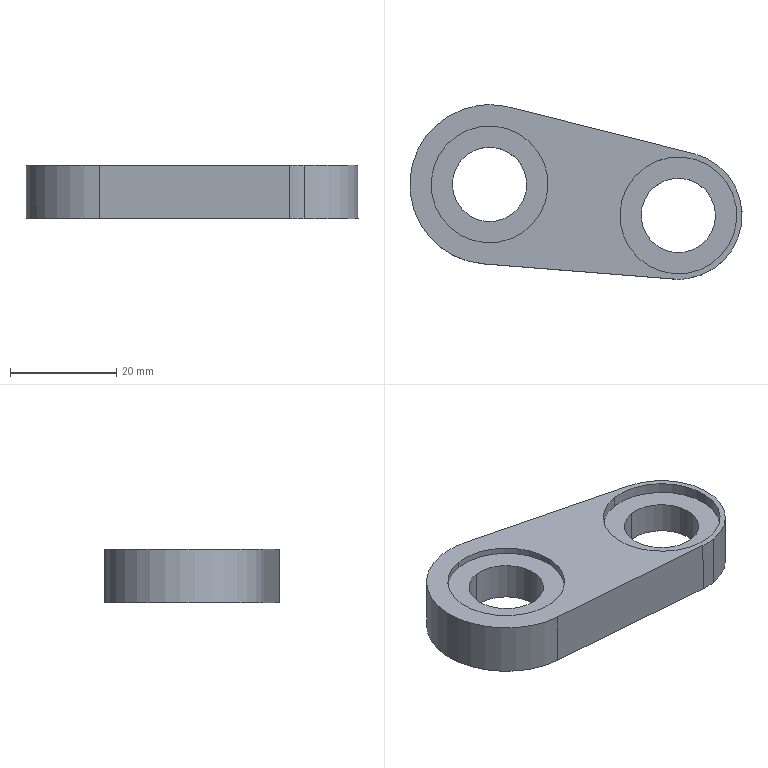Part | SolidWorks | features BaseBody 1 | 1 solid | 24 faces | box 62.525 x 32.838 x 10.009 mm | volume 10933 mm3 | cylinder 16 | plane 8 | commonest cylinder face diameters 22 x8 14 x4 24 x2 30 x2
STEP:
#1=CARTESIAN_POINT('',(378.377,184.65,13.48));
#2=VERTEX_POINT('',#1);
#3=CARTESIAN_POINT('',(376.21,198.481,13.48));
#4=VERTEX_POINT('',#3);
#5=CARTESIAN_POINT('',(377.293,191.566,13.48));
#6=DIRECTION('',(0.0001435,0.000000521,-1.));
#7=DIRECTION('',(1.,0.,0.0001435));
#8=AXIS2_PLACEMENT_3D('',#5,#6,#7);
#9=CIRCLE('',#8,7.);
#10=EDGE_CURVE('',#2,#4,#9,.T.);
#11=ORIENTED_EDGE('',*,*,#10,.F.);
#12=CARTESIAN_POINT('',(378.377,184.65,7.48));
#13=VERTEX_POINT('',#12);
#14=CARTESIAN_POINT('',(378.376,184.65,15.48));
#15=DIRECTION('',(0.0001435,0.000000521,-1.));
#16=VECTOR('',#15,1000.);
#17=LINE('',#14,#16);
#18=EDGE_CURVE('',#2,#13,#17,.T.);
#19=ORIENTED_EDGE('',*,*,#18,.T.);
#20=CARTESIAN_POINT('',(376.211,198.481,7.48));
#21=VERTEX_POINT('',#20);
#22=CARTESIAN_POINT('',(377.294,191.566,7.48));
#23=DIRECTION('',(-0.0001435,-0.000000521,1.));
#24=DIRECTION('',(0.1548,-0.988,0.00002169));
#25=AXIS2_PLACEMENT_3D('',#22,#23,#24);
#26=CIRCLE('',#25,7.);
#27=EDGE_CURVE('',#21,#13,#26,.T.);
#28=ORIENTED_EDGE('',*,*,#27,.F.);
#29=CARTESIAN_POINT('',(376.21,198.481,15.48));
#30=DIRECTION('',(0.0001435,0.000000521,-1.));
#31=VECTOR('',#30,1000.);
#32=LINE('',#29,#31);
#33=EDGE_CURVE('',#4,#21,#32,.T.);
#34=ORIENTED_EDGE('',*,*,#33,.F.);
#35=EDGE_LOOP('',(#11,#19,#28,#34));
#36=FACE_OUTER_BOUND('',#35,.T.);
#37=CARTESIAN_POINT('',(377.293,191.566,15.48));
#38=DIRECTION('',(0.0001435,0.000000521,-1.));
#39=DIRECTION('',(-0.1548,0.988,-0.00002169));
#40=AXIS2_PLACEMENT_3D('',#37,#38,#39);
#41=CYLINDRICAL_SURFACE('',#40,7.);
#42=ADVANCED_FACE('',(#36),#41,.F.);
#43=CARTESIAN_POINT('',(375.591,202.433,13.479));
#44=VERTEX_POINT('',#43);
#45=CARTESIAN_POINT('',(378.996,180.698,13.48));
#46=VERTEX_POINT('',#45);
#47=CARTESIAN_POINT('',(377.293,191.566,13.48));
#48=DIRECTION('',(-0.0001435,-0.000000521,1.));
#49=DIRECTION('',(0.1548,-0.988,0.00002169));
#50=AXIS2_PLACEMENT_3D('',#47,#48,#49);
#51=CIRCLE('',#50,11.);
#52=EDGE_CURVE('',#44,#46,#51,.T.);
#53=ORIENTED_EDGE('',*,*,#52,.F.);
#54=CARTESIAN_POINT('',(375.59,202.433,15.479));
#55=VERTEX_POINT('',#54);
#56=CARTESIAN_POINT('',(375.591,202.433,14.279));
#57=DIRECTION('',(-0.0001435,-0.000000521,1.));
#58=VECTOR('',#57,1000.);
#59=LINE('',#56,#58);
#60=EDGE_CURVE('',#44,#55,#59,.T.);
#61=ORIENTED_EDGE('',*,*,#60,.T.);
#62=CARTESIAN_POINT('',(378.995,180.698,15.48));
#63=VERTEX_POINT('',#62);
#64=CARTESIAN_POINT('',(377.293,191.566,15.48));
#65=DIRECTION('',(0.0001435,0.000000521,-1.));
#66=DIRECTION('',(-1.,0.,-0.0001435));
#67=AXIS2_PLACEMENT_3D('',#64,#65,#66);
#68=CIRCLE('',#67,11.);
#69=EDGE_CURVE('',#63,#55,#68,.T.);
#70=ORIENTED_EDGE('',*,*,#69,.F.);
#71=CARTESIAN_POINT('',(378.996,180.698,14.28));
#72=DIRECTION('',(-0.0001435,-0.000000521,1.));
#73=VECTOR('',#72,1000.);
#74=LINE('',#71,#73);
#75=EDGE_CURVE('',#46,#63,#74,.T.);
#76=ORIENTED_EDGE('',*,*,#75,.F.);
#77=EDGE_LOOP('',(#53,#61,#70,#76));
#78=FACE_OUTER_BOUND('',#77,.T.);
#79=CARTESIAN_POINT('',(377.293,191.566,14.28));
#80=DIRECTION('',(-0.0001435,-0.000000521,1.));
#81=DIRECTION('',(0.1548,-0.988,0.00002169));
#82=AXIS2_PLACEMENT_3D('',#79,#80,#81);
#83=CYLINDRICAL_SURFACE('',#82,11.);
#84=ADVANCED_FACE('',(#78),#83,.F.);
#85=CARTESIAN_POINT('',(340.067,208.271,14.274));
#86=VERTEX_POINT('',#85);
#87=CARTESIAN_POINT('',(343.472,186.536,14.275));
#88=VERTEX_POINT('',#87);
#89=CARTESIAN_POINT('',(341.77,197.404,14.275));
#90=DIRECTION('',(-0.0001435,-0.000000521,1.));
#91=DIRECTION('',(1.,0.,0.0001435));
#92=AXIS2_PLACEMENT_3D('',#89,#90,#91);
#93=CIRCLE('',#92,11.);
#94=EDGE_CURVE('',#86,#88,#93,.T.);
#95=ORIENTED_EDGE('',*,*,#94,.F.);
#96=CARTESIAN_POINT('',(340.067,208.271,15.474));
#97=VERTEX_POINT('',#96);
#98=CARTESIAN_POINT('',(340.067,208.271,14.274));
#99=DIRECTION('',(-0.0001435,-0.000000521,1.));
#100=VECTOR('',#99,1000.);
#101=LINE('',#98,#100);
#102=EDGE_CURVE('',#86,#97,#101,.T.);
#103=ORIENTED_EDGE('',*,*,#102,.T.);
#104=CARTESIAN_POINT('',(343.472,186.536,15.475));
#105=VERTEX_POINT('',#104);
#106=CARTESIAN_POINT('',(341.769,197.404,15.475));
#107=DIRECTION('',(0.0001435,0.000000521,-1.));
#108=DIRECTION('',(0.1548,-0.988,0.00002169));
#109=AXIS2_PLACEMENT_3D('',#106,#107,#108);
#110=CIRCLE('',#109,11.);
#111=EDGE_CURVE('',#105,#97,#110,.T.);
#112=ORIENTED_EDGE('',*,*,#111,.F.);
#113=CARTESIAN_POINT('',(343.472,186.536,14.275));
#114=DIRECTION('',(-0.0001435,-0.000000521,1.));
#115=VECTOR('',#114,1000.);
#116=LINE('',#113,#115);
#117=EDGE_CURVE('',#88,#105,#116,.T.);
#118=ORIENTED_EDGE('',*,*,#117,.F.);
#119=EDGE_LOOP('',(#95,#103,#112,#118));
#120=FACE_OUTER_BOUND('',#119,.T.);
#121=CARTESIAN_POINT('',(341.77,197.404,14.275));
#122=DIRECTION('',(-0.0001435,-0.000000521,1.));
#123=DIRECTION('',(0.1548,-0.988,0.00002169));
#124=AXIS2_PLACEMENT_3D('',#121,#122,#123);
#125=CYLINDRICAL_SURFACE('',#124,11.);
#126=ADVANCED_FACE('',(#120),#125,.F.);
#127=CARTESIAN_POINT('',(342.853,190.488,14.275));
#128=VERTEX_POINT('',#127);
#129=CARTESIAN_POINT('',(340.686,204.319,14.274));
#130=VERTEX_POINT('',#129);
#131=CARTESIAN_POINT('',(341.77,197.404,14.275));
#132=DIRECTION('',(0.0001435,0.000000521,-1.));
#133=DIRECTION('',(-0.1548,0.988,-0.00002169));
#134=AXIS2_PLACEMENT_3D('',#131,#132,#133);
#135=CIRCLE('',#134,7.);
#136=EDGE_CURVE('',#128,#130,#135,.T.);
#137=ORIENTED_EDGE('',*,*,#136,.F.);
#138=CARTESIAN_POINT('',(342.854,190.488,7.075));
#139=VERTEX_POINT('',#138);
#140=CARTESIAN_POINT('',(342.853,190.488,14.275));
#141=DIRECTION('',(0.0001435,0.000000521,-1.));
#142=VECTOR('',#141,1000.);
#143=LINE('',#140,#142);
#144=EDGE_CURVE('',#128,#139,#143,.T.);
#145=ORIENTED_EDGE('',*,*,#144,.T.);
#146=CARTESIAN_POINT('',(340.687,204.319,7.074));
#147=VERTEX_POINT('',#146);
#148=CARTESIAN_POINT('',(341.771,197.404,7.075));
#149=DIRECTION('',(-0.0001435,-0.000000521,1.));
#150=DIRECTION('',(-0.1548,0.988,-0.00002169));
#151=AXIS2_PLACEMENT_3D('',#148,#149,#150);
#152=CIRCLE('',#151,7.);
#153=EDGE_CURVE('',#147,#139,#152,.T.);
#154=ORIENTED_EDGE('',*,*,#153,.F.);
#155=CARTESIAN_POINT('',(340.686,204.319,14.274));
#156=DIRECTION('',(0.0001435,0.000000521,-1.));
#157=VECTOR('',#156,1000.);
#158=LINE('',#155,#157);
#159=EDGE_CURVE('',#130,#147,#158,.T.);
#160=ORIENTED_EDGE('',*,*,#159,.F.);
#161=EDGE_LOOP('',(#137,#145,#154,#160));
#162=FACE_OUTER_BOUND('',#161,.T.);
#163=CARTESIAN_POINT('',(341.77,197.404,14.275));
#164=DIRECTION('',(0.0001435,0.000000521,-1.));
#165=DIRECTION('',(-0.1548,0.988,-0.00002169));
#166=AXIS2_PLACEMENT_3D('',#163,#164,#165);
#167=CYLINDRICAL_SURFACE('',#166,7.);
#168=ADVANCED_FACE('',(#162),#167,.F.);
#169=CARTESIAN_POINT('',(340.068,208.271,7.074));
#170=VERTEX_POINT('',#169);
#171=CARTESIAN_POINT('',(343.473,186.536,7.075));
#172=VERTEX_POINT('',#171);
#173=CARTESIAN_POINT('',(341.771,197.404,7.075));
#174=DIRECTION('',(0.0001435,0.000000521,-1.));
#175=DIRECTION('',(-0.1548,0.988,-0.00002169));
#176=AXIS2_PLACEMENT_3D('',#173,#174,#175);
#177=CIRCLE('',#176,11.);
#178=EDGE_CURVE('',#170,#172,#177,.T.);
#179=ORIENTED_EDGE('',*,*,#178,.F.);
#180=CARTESIAN_POINT('',(340.068,208.271,5.474));
#181=VERTEX_POINT('',#180);
#182=CARTESIAN_POINT('',(340.068,208.271,7.074));
#183=DIRECTION('',(0.0001435,0.000000521,-1.));
#184=VECTOR('',#183,1000.);
#185=LINE('',#182,#184);
#186=EDGE_CURVE('',#170,#181,#185,.T.);
#187=ORIENTED_EDGE('',*,*,#186,.T.);
#188=CARTESIAN_POINT('',(343.473,186.536,5.475));
#189=VERTEX_POINT('',#188);
#190=CARTESIAN_POINT('',(341.771,197.404,5.475));
#191=DIRECTION('',(-0.0001435,-0.000000521,1.));
#192=DIRECTION('',(-1.,0.,-0.0001435));
#193=AXIS2_PLACEMENT_3D('',#190,#191,#192);
#194=CIRCLE('',#193,11.);
#195=EDGE_CURVE('',#189,#181,#194,.T.);
#196=ORIENTED_EDGE('',*,*,#195,.F.);
#197=CARTESIAN_POINT('',(343.473,186.536,7.075));
#198=DIRECTION('',(0.0001435,0.000000521,-1.));
#199=VECTOR('',#198,1000.);
#200=LINE('',#197,#199);
#201=EDGE_CURVE('',#172,#189,#200,.T.);
#202=ORIENTED_EDGE('',*,*,#201,.F.);
#203=EDGE_LOOP('',(#179,#187,#196,#202));
#204=FACE_OUTER_BOUND('',#203,.T.);
#205=CARTESIAN_POINT('',(341.771,197.404,7.075));
#206=DIRECTION('',(0.0001435,0.000000521,-1.));
#207=DIRECTION('',(0.1548,-0.988,0.00002169));
#208=AXIS2_PLACEMENT_3D('',#205,#206,#207);
#209=CYLINDRICAL_SURFACE('',#208,11.);
#210=ADVANCED_FACE('',(#204),#209,.F.);
#211=CARTESIAN_POINT('',(375.592,202.433,7.479));
#212=VERTEX_POINT('',#211);
#213=CARTESIAN_POINT('',(378.997,180.698,7.48));
#214=VERTEX_POINT('',#213);
#215=CARTESIAN_POINT('',(377.294,191.566,7.48));
#216=DIRECTION('',(0.0001435,0.000000521,-1.));
#217=DIRECTION('',(-0.1548,0.988,-0.00002169));
#218=AXIS2_PLACEMENT_3D('',#215,#216,#217);
#219=CIRCLE('',#218,11.);
#220=EDGE_CURVE('',#212,#214,#219,.T.);
#221=ORIENTED_EDGE('',*,*,#220,.F.);
#222=CARTESIAN_POINT('',(375.592,202.433,5.479));
#223=VERTEX_POINT('',#222);
#224=CARTESIAN_POINT('',(375.592,202.433,7.079));
#225=DIRECTION('',(0.0001435,0.000000521,-1.));
#226=VECTOR('',#225,1000.);
#227=LINE('',#224,#226);
#228=EDGE_CURVE('',#212,#223,#227,.T.);
#229=ORIENTED_EDGE('',*,*,#228,.T.);
#230=CARTESIAN_POINT('',(378.997,180.698,5.48));
#231=VERTEX_POINT('',#230);
#232=CARTESIAN_POINT('',(377.294,191.566,5.48));
#233=DIRECTION('',(-0.0001435,-0.000000521,1.));
#234=DIRECTION('',(0.1548,-0.988,0.00002169));
#235=AXIS2_PLACEMENT_3D('',#232,#233,#234);
#236=CIRCLE('',#235,11.);
#237=EDGE_CURVE('',#231,#223,#236,.T.);
#238=ORIENTED_EDGE('',*,*,#237,.F.);
#239=CARTESIAN_POINT('',(378.997,180.698,7.08));
#240=DIRECTION('',(0.0001435,0.000000521,-1.));
#241=VECTOR('',#240,1000.);
#242=LINE('',#239,#241);
#243=EDGE_CURVE('',#214,#231,#242,.T.);
#244=ORIENTED_EDGE('',*,*,#243,.F.);
#245=EDGE_LOOP('',(#221,#229,#238,#244));
#246=FACE_OUTER_BOUND('',#245,.T.);
#247=CARTESIAN_POINT('',(377.294,191.566,7.08));
#248=DIRECTION('',(0.0001435,0.000000521,-1.));
#249=DIRECTION('',(0.1548,-0.988,0.00002169));
#250=AXIS2_PLACEMENT_3D('',#247,#248,#249);
#251=CYLINDRICAL_SURFACE('',#250,11.);
#252=ADVANCED_FACE('',(#246),#251,.F.);
#253=CARTESIAN_POINT('',(379.152,179.71,5.48));
#254=VERTEX_POINT('',#253);
#255=CARTESIAN_POINT('',(376.342,179.604,5.48));
#256=VERTEX_POINT('',#255);
#257=CARTESIAN_POINT('',(377.294,191.566,5.48));
#258=DIRECTION('',(0.0001435,0.000000521,-1.));
#259=DIRECTION('',(0.1548,-0.988,0.00002169));
#260=AXIS2_PLACEMENT_3D('',#257,#258,#259);
#261=CIRCLE('',#260,12.);
#262=EDGE_CURVE('',#254,#256,#261,.T.);
#263=ORIENTED_EDGE('',*,*,#262,.F.);
#264=CARTESIAN_POINT('',(379.15,179.71,15.48));
#265=VERTEX_POINT('',#264);
#266=CARTESIAN_POINT('',(379.15,179.71,15.48));
#267=DIRECTION('',(-0.0001435,-0.000000521,1.));
#268=VECTOR('',#267,1000.);
#269=LINE('',#266,#268);
#270=EDGE_CURVE('',#254,#265,#269,.T.);
#271=ORIENTED_EDGE('',*,*,#270,.T.);
#272=CARTESIAN_POINT('',(376.341,179.604,15.48));
#273=VERTEX_POINT('',#272);
#274=CARTESIAN_POINT('',(377.293,191.566,15.48));
#275=DIRECTION('',(-0.0001435,-0.000000521,1.));
#276=DIRECTION('',(-0.07937,-0.9968,-0.00001191));
#277=AXIS2_PLACEMENT_3D('',#274,#275,#276);
#278=CIRCLE('',#277,12.);
#279=EDGE_CURVE('',#273,#265,#278,.T.);
#280=ORIENTED_EDGE('',*,*,#279,.F.);
#281=CARTESIAN_POINT('',(376.341,179.604,15.48));
#282=DIRECTION('',(0.0001435,0.000000521,-1.));
#283=VECTOR('',#282,1000.);
#284=LINE('',#281,#283);
#285=EDGE_CURVE('',#273,#256,#284,.T.);
#286=ORIENTED_EDGE('',*,*,#285,.T.);
#287=EDGE_LOOP('',(#263,#271,#280,#286));
#288=FACE_OUTER_BOUND('',#287,.T.);
#289=CARTESIAN_POINT('',(377.293,191.566,15.48));
#290=DIRECTION('',(-0.0001435,-0.000000521,1.));
#291=DIRECTION('',(0.1548,-0.988,0.00002169));
#292=AXIS2_PLACEMENT_3D('',#289,#290,#291);
#293=CYLINDRICAL_SURFACE('',#292,12.);
#294=ADVANCED_FACE('',(#288),#293,.T.);
#295=CARTESIAN_POINT('',(339.448,212.223,15.474));
#296=VERTEX_POINT('',#295);
#297=CARTESIAN_POINT('',(340.579,182.451,15.474));
#298=VERTEX_POINT('',#297);
#299=CARTESIAN_POINT('',(341.769,197.404,15.475));
#300=DIRECTION('',(-0.0001435,-0.000000521,1.));
#301=DIRECTION('',(0.2438,0.9698,0.00003549));
#302=AXIS2_PLACEMENT_3D('',#299,#300,#301);
#303=CIRCLE('',#302,15.);
#304=EDGE_CURVE('',#296,#298,#303,.T.);
#305=ORIENTED_EDGE('',*,*,#304,.F.);
#306=CARTESIAN_POINT('',(339.449,212.223,5.474));
#307=VERTEX_POINT('',#306);
#308=CARTESIAN_POINT('',(339.448,212.223,15.474));
#309=DIRECTION('',(0.0001435,0.000000521,-1.));
#310=VECTOR('',#309,1000.);
#311=LINE('',#308,#310);
#312=EDGE_CURVE('',#296,#307,#311,.T.);
#313=ORIENTED_EDGE('',*,*,#312,.T.);
#314=CARTESIAN_POINT('',(340.58,182.451,5.474));
#315=VERTEX_POINT('',#314);
#316=CARTESIAN_POINT('',(341.771,197.404,5.475));
#317=DIRECTION('',(0.0001435,0.000000521,-1.));
#318=DIRECTION('',(-0.07937,-0.9968,-0.00001191));
#319=AXIS2_PLACEMENT_3D('',#316,#317,#318);
#320=CIRCLE('',#319,15.);
#321=EDGE_CURVE('',#315,#307,#320,.T.);
#322=ORIENTED_EDGE('',*,*,#321,.F.);
#323=CARTESIAN_POINT('',(340.58,182.451,5.474));
#324=DIRECTION('',(-0.0001435,-0.000000521,1.));
#325=VECTOR('',#324,1000.);
#326=LINE('',#323,#325);
#327=EDGE_CURVE('',#315,#298,#326,.T.);
#328=ORIENTED_EDGE('',*,*,#327,.T.);
#329=EDGE_LOOP('',(#305,#313,#322,#328));
#330=FACE_OUTER_BOUND('',#329,.T.);
#331=CARTESIAN_POINT('',(341.769,197.404,15.475));
#332=DIRECTION('',(0.0001435,0.000000521,-1.));
#333=DIRECTION('',(-0.1548,0.988,-0.00002169));
#334=AXIS2_PLACEMENT_3D('',#331,#332,#333);
#335=CYLINDRICAL_SURFACE('',#334,15.);
#336=ADVANCED_FACE('',(#330),#335,.T.);
#337=ORIENTED_EDGE('',*,*,#285,.F.);
#338=CARTESIAN_POINT('',(340.579,182.451,15.474));
#339=DIRECTION('',(0.9968,-0.07937,0.000143));
#340=VECTOR('',#339,1000.);
#341=LINE('',#338,#340);
#342=EDGE_CURVE('',#298,#273,#341,.T.);
#343=ORIENTED_EDGE('',*,*,#342,.F.);
#344=ORIENTED_EDGE('',*,*,#327,.F.);
#345=CARTESIAN_POINT('',(376.342,179.604,5.48));
#346=DIRECTION('',(-0.9968,0.07937,-0.000143));
#347=VECTOR('',#346,1000.);
#348=LINE('',#345,#347);
#349=EDGE_CURVE('',#256,#315,#348,.T.);
#350=ORIENTED_EDGE('',*,*,#349,.F.);
#351=EDGE_LOOP('',(#337,#343,#344,#350));
#352=FACE_OUTER_BOUND('',#351,.T.);
#353=CARTESIAN_POINT('',(340.58,182.451,15.474));
#354=DIRECTION('',(-0.07937,-0.9968,-0.00001191));
#355=DIRECTION('',(-0.9968,0.07937,0.));
#356=AXIS2_PLACEMENT_3D('',#353,#354,#355);
#357=PLANE('',#356);
#358=ADVANCED_FACE('',(#352),#357,.T.);
#359=ORIENTED_EDGE('',*,*,#312,.F.);
#360=CARTESIAN_POINT('',(345.427,211.951,15.475));
#361=VERTEX_POINT('',#360);
#362=CARTESIAN_POINT('',(341.769,197.404,15.475));
#363=DIRECTION('',(-0.0001435,-0.000000521,1.));
#364=DIRECTION('',(0.2438,0.9698,0.00003549));
#365=AXIS2_PLACEMENT_3D('',#362,#363,#364);
#366=CIRCLE('',#365,15.);
#367=EDGE_CURVE('',#361,#296,#366,.T.);
#368=ORIENTED_EDGE('',*,*,#367,.F.);
#369=CARTESIAN_POINT('',(345.428,211.951,5.475));
#370=VERTEX_POINT('',#369);
#371=CARTESIAN_POINT('',(345.427,211.951,15.475));
#372=DIRECTION('',(0.0001435,0.000000522,-1.));
#373=VECTOR('',#372,1000.);
#374=LINE('',#371,#373);
#375=EDGE_CURVE('',#361,#370,#374,.T.);
#376=ORIENTED_EDGE('',*,*,#375,.T.);
#377=CARTESIAN_POINT('',(341.771,197.404,5.475));
#378=DIRECTION('',(0.0001435,0.000000521,-1.));
#379=DIRECTION('',(-0.07937,-0.9968,-0.00001191));
#380=AXIS2_PLACEMENT_3D('',#377,#378,#379);
#381=CIRCLE('',#380,15.);
#382=EDGE_CURVE('',#307,#370,#381,.T.);
#383=ORIENTED_EDGE('',*,*,#382,.F.);
#384=EDGE_LOOP('',(#359,#368,#376,#383));
#385=FACE_OUTER_BOUND('',#384,.T.);
#386=CARTESIAN_POINT('',(341.769,197.404,15.475));
#387=DIRECTION('',(0.0001435,0.000000521,-1.));
#388=DIRECTION('',(-0.1548,0.988,-0.00002169));
#389=AXIS2_PLACEMENT_3D('',#386,#387,#388);
#390=CYLINDRICAL_SURFACE('',#389,15.);
#391=ADVANCED_FACE('',(#385),#390,.T.);
#392=ORIENTED_EDGE('',*,*,#375,.F.);
#393=CARTESIAN_POINT('',(380.219,203.204,15.48));
#394=VERTEX_POINT('',#393);
#395=CARTESIAN_POINT('',(380.219,203.204,15.48));
#396=DIRECTION('',(-0.9698,0.2438,-0.000139));
#397=VECTOR('',#396,1000.);
#398=LINE('',#395,#397);
#399=EDGE_CURVE('',#394,#361,#398,.T.);
#400=ORIENTED_EDGE('',*,*,#399,.F.);
#401=CARTESIAN_POINT('',(380.22,203.204,5.48));
#402=VERTEX_POINT('',#401);
#403=CARTESIAN_POINT('',(380.22,203.204,5.48));
#404=DIRECTION('',(-0.0001435,-0.000000521,1.));
#405=VECTOR('',#404,1000.);
#406=LINE('',#403,#405);
#407=EDGE_CURVE('',#402,#394,#406,.T.);
#408=ORIENTED_EDGE('',*,*,#407,.F.);
#409=CARTESIAN_POINT('',(345.428,211.951,5.475));
#410=DIRECTION('',(0.9698,-0.2438,0.000139));
#411=VECTOR('',#410,1000.);
#412=LINE('',#409,#411);
#413=EDGE_CURVE('',#370,#402,#412,.T.);
#414=ORIENTED_EDGE('',*,*,#413,.F.);
#415=EDGE_LOOP('',(#392,#400,#408,#414));
#416=FACE_OUTER_BOUND('',#415,.T.);
#417=CARTESIAN_POINT('',(345.428,211.951,15.475));
#418=DIRECTION('',(0.2438,0.9698,0.00003549));
#419=DIRECTION('',(0.0001455,0.,-1.));
#420=AXIS2_PLACEMENT_3D('',#417,#418,#419);
#421=PLANE('',#420);
#422=ADVANCED_FACE('',(#416),#421,.T.);
#423=ORIENTED_EDGE('',*,*,#270,.F.);
#424=CARTESIAN_POINT('',(377.294,191.566,5.48));
#425=DIRECTION('',(0.0001435,0.000000521,-1.));
#426=DIRECTION('',(0.1548,-0.988,0.00002169));
#427=AXIS2_PLACEMENT_3D('',#424,#425,#426);
#428=CIRCLE('',#427,12.);
#429=EDGE_CURVE('',#402,#254,#428,.T.);
#430=ORIENTED_EDGE('',*,*,#429,.F.);
#431=ORIENTED_EDGE('',*,*,#407,.T.);
#432=CARTESIAN_POINT('',(377.293,191.566,15.48));
#433=DIRECTION('',(-0.0001435,-0.000000521,1.));
#434=DIRECTION('',(-0.07937,-0.9968,-0.00001191));
#435=AXIS2_PLACEMENT_3D('',#432,#433,#434);
#436=CIRCLE('',#435,12.);
#437=EDGE_CURVE('',#265,#394,#436,.T.);
#438=ORIENTED_EDGE('',*,*,#437,.F.);
#439=EDGE_LOOP('',(#423,#430,#431,#438));
#440=FACE_OUTER_BOUND('',#439,.T.);
#441=CARTESIAN_POINT('',(377.293,191.566,15.48));
#442=DIRECTION('',(-0.0001435,-0.000000521,1.));
#443=DIRECTION('',(0.1548,-0.988,0.00002169));
#444=AXIS2_PLACEMENT_3D('',#441,#442,#443);
#445=CYLINDRICAL_SURFACE('',#444,12.);
#446=ADVANCED_FACE('',(#440),#445,.T.);
#447=ORIENTED_EDGE('',*,*,#228,.F.);
#448=CARTESIAN_POINT('',(377.294,191.566,7.48));
#449=DIRECTION('',(0.0001435,0.000000521,-1.));
#450=DIRECTION('',(-0.1548,0.988,-0.00002169));
#451=AXIS2_PLACEMENT_3D('',#448,#449,#450);
#452=CIRCLE('',#451,11.);
#453=EDGE_CURVE('',#214,#212,#452,.T.);
#454=ORIENTED_EDGE('',*,*,#453,.F.);
#455=ORIENTED_EDGE('',*,*,#243,.T.);
#456=CARTESIAN_POINT('',(377.294,191.566,5.48));
#457=DIRECTION('',(-0.0001435,-0.000000521,1.));
#458=DIRECTION('',(0.1548,-0.988,0.00002169));
#459=AXIS2_PLACEMENT_3D('',#456,#457,#458);
#460=CIRCLE('',#459,11.);
#461=EDGE_CURVE('',#223,#231,#460,.T.);
#462=ORIENTED_EDGE('',*,*,#461,.F.);
#463=EDGE_LOOP('',(#447,#454,#455,#462));
#464=FACE_OUTER_BOUND('',#463,.T.);
#465=CARTESIAN_POINT('',(377.294,191.566,7.08));
#466=DIRECTION('',(0.0001435,0.000000521,-1.));
#467=DIRECTION('',(0.1548,-0.988,0.00002169));
#468=AXIS2_PLACEMENT_3D('',#465,#466,#467);
#469=CYLINDRICAL_SURFACE('',#468,11.);
#470=ADVANCED_FACE('',(#464),#469,.F.);
#471=ORIENTED_EDGE('',*,*,#237,.T.);
#472=ORIENTED_EDGE('',*,*,#461,.T.);
#473=EDGE_LOOP('',(#471,#472));
#474=FACE_BOUND('',#473,.T.);
#475=ORIENTED_EDGE('',*,*,#195,.T.);
#476=CARTESIAN_POINT('',(341.771,197.404,5.475));
#477=DIRECTION('',(-0.0001435,-0.000000521,1.));
#478=DIRECTION('',(-1.,0.,-0.0001435));
#479=AXIS2_PLACEMENT_3D('',#476,#477,#478);
#480=CIRCLE('',#479,11.);
#481=EDGE_CURVE('',#181,#189,#480,.T.);
#482=ORIENTED_EDGE('',*,*,#481,.T.);
#483=EDGE_LOOP('',(#475,#482));
#484=FACE_BOUND('',#483,.T.);
#485=ORIENTED_EDGE('',*,*,#429,.T.);
#486=ORIENTED_EDGE('',*,*,#262,.T.);
#487=ORIENTED_EDGE('',*,*,#349,.T.);
#488=ORIENTED_EDGE('',*,*,#321,.T.);
#489=ORIENTED_EDGE('',*,*,#382,.T.);
#490=ORIENTED_EDGE('',*,*,#413,.T.);
#491=EDGE_LOOP('',(#485,#486,#487,#488,#489,#490));
#492=FACE_OUTER_BOUND('',#491,.T.);
#493=CARTESIAN_POINT('',(377.294,191.566,5.48));
#494=DIRECTION('',(0.0001435,0.000000521,-1.));
#495=DIRECTION('',(0.,-1.,-0.000000521));
#496=AXIS2_PLACEMENT_3D('',#493,#494,#495);
#497=PLANE('',#496);
#498=ADVANCED_FACE('',(#474,#484,#492),#497,.T.);
#499=ORIENTED_EDGE('',*,*,#186,.F.);
#500=CARTESIAN_POINT('',(341.771,197.404,7.075));
#501=DIRECTION('',(0.0001435,0.000000521,-1.));
#502=DIRECTION('',(-0.1548,0.988,-0.00002169));
#503=AXIS2_PLACEMENT_3D('',#500,#501,#502);
#504=CIRCLE('',#503,11.);
#505=EDGE_CURVE('',#172,#170,#504,.T.);
#506=ORIENTED_EDGE('',*,*,#505,.F.);
#507=ORIENTED_EDGE('',*,*,#201,.T.);
#508=ORIENTED_EDGE('',*,*,#481,.F.);
#509=EDGE_LOOP('',(#499,#506,#507,#508));
#510=FACE_OUTER_BOUND('',#509,.T.);
#511=CARTESIAN_POINT('',(341.771,197.404,7.075));
#512=DIRECTION('',(0.0001435,0.000000521,-1.));
#513=DIRECTION('',(0.1548,-0.988,0.00002169));
#514=AXIS2_PLACEMENT_3D('',#511,#512,#513);
#515=CYLINDRICAL_SURFACE('',#514,11.);
#516=ADVANCED_FACE('',(#510),#515,.F.);
#517=ORIENTED_EDGE('',*,*,#153,.T.);
#518=CARTESIAN_POINT('',(341.771,197.404,7.075));
#519=DIRECTION('',(-0.0001435,-0.000000521,1.));
#520=DIRECTION('',(-0.1548,0.988,-0.00002169));
#521=AXIS2_PLACEMENT_3D('',#518,#519,#520);
#522=CIRCLE('',#521,7.);
#523=EDGE_CURVE('',#139,#147,#522,.T.);
#524=ORIENTED_EDGE('',*,*,#523,.T.);
#525=EDGE_LOOP('',(#517,#524));
#526=FACE_BOUND('',#525,.T.);
#527=ORIENTED_EDGE('',*,*,#505,.T.);
#528=ORIENTED_EDGE('',*,*,#178,.T.);
#529=EDGE_LOOP('',(#527,#528));
#530=FACE_OUTER_BOUND('',#529,.T.);
#531=CARTESIAN_POINT('',(341.771,197.404,7.075));
#532=DIRECTION('',(-0.0001435,-0.000000521,1.));
#533=DIRECTION('',(-0.003633,1.,0.));
#534=AXIS2_PLACEMENT_3D('',#531,#532,#533);
#535=PLANE('',#534);
#536=ADVANCED_FACE('',(#526,#530),#535,.F.);
#537=ORIENTED_EDGE('',*,*,#144,.F.);
#538=CARTESIAN_POINT('',(341.77,197.404,14.275));
#539=DIRECTION('',(0.0001435,0.000000521,-1.));
#540=DIRECTION('',(-0.1548,0.988,-0.00002169));
#541=AXIS2_PLACEMENT_3D('',#538,#539,#540);
#542=CIRCLE('',#541,7.);
#543=EDGE_CURVE('',#130,#128,#542,.T.);
#544=ORIENTED_EDGE('',*,*,#543,.F.);
#545=ORIENTED_EDGE('',*,*,#159,.T.);
#546=ORIENTED_EDGE('',*,*,#523,.F.);
#547=EDGE_LOOP('',(#537,#544,#545,#546));
#548=FACE_OUTER_BOUND('',#547,.T.);
#549=CARTESIAN_POINT('',(341.77,197.404,14.275));
#550=DIRECTION('',(0.0001435,0.000000521,-1.));
#551=DIRECTION('',(-0.1548,0.988,-0.00002169));
#552=AXIS2_PLACEMENT_3D('',#549,#550,#551);
#553=CYLINDRICAL_SURFACE('',#552,7.);
#554=ADVANCED_FACE('',(#548),#553,.F.);
#555=ORIENTED_EDGE('',*,*,#543,.T.);
#556=ORIENTED_EDGE('',*,*,#136,.T.);
#557=EDGE_LOOP('',(#555,#556));
#558=FACE_BOUND('',#557,.T.);
#559=CARTESIAN_POINT('',(341.77,197.404,14.275));
#560=DIRECTION('',(-0.0001435,-0.000000521,1.));
#561=DIRECTION('',(1.,0.,0.0001435));
#562=AXIS2_PLACEMENT_3D('',#559,#560,#561);
#563=CIRCLE('',#562,11.);
#564=EDGE_CURVE('',#88,#86,#563,.T.);
#565=ORIENTED_EDGE('',*,*,#564,.T.);
#566=ORIENTED_EDGE('',*,*,#94,.T.);
#567=EDGE_LOOP('',(#565,#566));
#568=FACE_OUTER_BOUND('',#567,.T.);
#569=CARTESIAN_POINT('',(341.77,197.404,14.275));
#570=DIRECTION('',(0.0001435,0.000000521,-1.));
#571=DIRECTION('',(0.,-1.,-0.000000521));
#572=AXIS2_PLACEMENT_3D('',#569,#570,#571);
#573=PLANE('',#572);
#574=ADVANCED_FACE('',(#558,#568),#573,.F.);
#575=ORIENTED_EDGE('',*,*,#102,.F.);
#576=ORIENTED_EDGE('',*,*,#564,.F.);
#577=ORIENTED_EDGE('',*,*,#117,.T.);
#578=CARTESIAN_POINT('',(341.769,197.404,15.475));
#579=DIRECTION('',(0.0001435,0.000000521,-1.));
#580=DIRECTION('',(0.1548,-0.988,0.00002169));
#581=AXIS2_PLACEMENT_3D('',#578,#579,#580);
#582=CIRCLE('',#581,11.);
#583=EDGE_CURVE('',#97,#105,#582,.T.);
#584=ORIENTED_EDGE('',*,*,#583,.F.);
#585=EDGE_LOOP('',(#575,#576,#577,#584));
#586=FACE_OUTER_BOUND('',#585,.T.);
#587=CARTESIAN_POINT('',(341.77,197.404,14.275));
#588=DIRECTION('',(-0.0001435,-0.000000521,1.));
#589=DIRECTION('',(0.1548,-0.988,0.00002169));
#590=AXIS2_PLACEMENT_3D('',#587,#588,#589);
#591=CYLINDRICAL_SURFACE('',#590,11.);
#592=ADVANCED_FACE('',(#586),#591,.F.);
#593=ORIENTED_EDGE('',*,*,#69,.T.);
#594=CARTESIAN_POINT('',(377.293,191.566,15.48));
#595=DIRECTION('',(0.0001435,0.000000521,-1.));
#596=DIRECTION('',(-1.,0.,-0.0001435));
#597=AXIS2_PLACEMENT_3D('',#594,#595,#596);
#598=CIRCLE('',#597,11.);
#599=EDGE_CURVE('',#55,#63,#598,.T.);
#600=ORIENTED_EDGE('',*,*,#599,.T.);
#601=EDGE_LOOP('',(#593,#600));
#602=FACE_BOUND('',#601,.T.);
#603=ORIENTED_EDGE('',*,*,#111,.T.);
#604=ORIENTED_EDGE('',*,*,#583,.T.);
#605=EDGE_LOOP('',(#603,#604));
#606=FACE_BOUND('',#605,.T.);
#607=ORIENTED_EDGE('',*,*,#342,.T.);
#608=ORIENTED_EDGE('',*,*,#279,.T.);
#609=ORIENTED_EDGE('',*,*,#437,.T.);
#610=ORIENTED_EDGE('',*,*,#399,.T.);
#611=ORIENTED_EDGE('',*,*,#367,.T.);
#612=ORIENTED_EDGE('',*,*,#304,.T.);
#613=EDGE_LOOP('',(#607,#608,#609,#610,#611,#612));
#614=FACE_OUTER_BOUND('',#613,.T.);
#615=CARTESIAN_POINT('',(377.293,191.566,15.48));
#616=DIRECTION('',(0.0001435,0.000000521,-1.));
#617=DIRECTION('',(0.,-1.,-0.000000521));
#618=AXIS2_PLACEMENT_3D('',#615,#616,#617);
#619=PLANE('',#618);
#620=ADVANCED_FACE('',(#602,#606,#614),#619,.F.);
#621=ORIENTED_EDGE('',*,*,#60,.F.);
#622=CARTESIAN_POINT('',(377.293,191.566,13.48));
#623=DIRECTION('',(-0.0001435,-0.000000521,1.));
#624=DIRECTION('',(0.1548,-0.988,0.00002169));
#625=AXIS2_PLACEMENT_3D('',#622,#623,#624);
#626=CIRCLE('',#625,11.);
#627=EDGE_CURVE('',#46,#44,#626,.T.);
#628=ORIENTED_EDGE('',*,*,#627,.F.);
#629=ORIENTED_EDGE('',*,*,#75,.T.);
#630=ORIENTED_EDGE('',*,*,#599,.F.);
#631=EDGE_LOOP('',(#621,#628,#629,#630));
#632=FACE_OUTER_BOUND('',#631,.T.);
#633=CARTESIAN_POINT('',(377.293,191.566,14.28));
#634=DIRECTION('',(-0.0001435,-0.000000521,1.));
#635=DIRECTION('',(0.1548,-0.988,0.00002169));
#636=AXIS2_PLACEMENT_3D('',#633,#634,#635);
#637=CYLINDRICAL_SURFACE('',#636,11.);
#638=ADVANCED_FACE('',(#632),#637,.F.);
#639=CARTESIAN_POINT('',(377.293,191.566,13.48));
#640=DIRECTION('',(0.0001435,0.000000521,-1.));
#641=DIRECTION('',(1.,0.,0.0001435));
#642=AXIS2_PLACEMENT_3D('',#639,#640,#641);
#643=CIRCLE('',#642,7.);
#644=EDGE_CURVE('',#4,#2,#643,.T.);
#645=ORIENTED_EDGE('',*,*,#644,.T.);
#646=ORIENTED_EDGE('',*,*,#10,.T.);
#647=EDGE_LOOP('',(#645,#646));
#648=FACE_BOUND('',#647,.T.);
#649=ORIENTED_EDGE('',*,*,#627,.T.);
#650=ORIENTED_EDGE('',*,*,#52,.T.);
#651=EDGE_LOOP('',(#649,#650));
#652=FACE_OUTER_BOUND('',#651,.T.);
#653=CARTESIAN_POINT('',(377.293,191.566,13.48));
#654=DIRECTION('',(0.0001435,0.000000521,-1.));
#655=DIRECTION('',(0.,-1.,-0.000000521));
#656=AXIS2_PLACEMENT_3D('',#653,#654,#655);
#657=PLANE('',#656);
#658=ADVANCED_FACE('',(#648,#652),#657,.F.);
#659=ORIENTED_EDGE('',*,*,#27,.T.);
#660=CARTESIAN_POINT('',(377.294,191.566,7.48));
#661=DIRECTION('',(-0.0001435,-0.000000521,1.));
#662=DIRECTION('',(0.1548,-0.988,0.00002169));
#663=AXIS2_PLACEMENT_3D('',#660,#661,#662);
#664=CIRCLE('',#663,7.);
#665=EDGE_CURVE('',#13,#21,#664,.T.);
#666=ORIENTED_EDGE('',*,*,#665,.T.);
#667=EDGE_LOOP('',(#659,#666));
#668=FACE_BOUND('',#667,.T.);
#669=ORIENTED_EDGE('',*,*,#453,.T.);
#670=ORIENTED_EDGE('',*,*,#220,.T.);
#671=EDGE_LOOP('',(#669,#670));
#672=FACE_OUTER_BOUND('',#671,.T.);
#673=CARTESIAN_POINT('',(377.294,191.566,7.48));
#674=DIRECTION('',(0.0001435,0.000000521,-1.));
#675=DIRECTION('',(0.,-1.,-0.000000521));
#676=AXIS2_PLACEMENT_3D('',#673,#674,#675);
#677=PLANE('',#676);
#678=ADVANCED_FACE('',(#668,#672),#677,.T.);
#679=ORIENTED_EDGE('',*,*,#18,.F.);
#680=ORIENTED_EDGE('',*,*,#644,.F.);
#681=ORIENTED_EDGE('',*,*,#33,.T.);
#682=ORIENTED_EDGE('',*,*,#665,.F.);
#683=EDGE_LOOP('',(#679,#680,#681,#682));
#684=FACE_OUTER_BOUND('',#683,.T.);
#685=CARTESIAN_POINT('',(377.293,191.566,15.48));
#686=DIRECTION('',(0.0001435,0.000000521,-1.));
#687=DIRECTION('',(-0.1548,0.988,-0.00002169));
#688=AXIS2_PLACEMENT_3D('',#685,#686,#687);
#689=CYLINDRICAL_SURFACE('',#688,7.);
#690=ADVANCED_FACE('',(#684),#689,.F.);
#691=CLOSED_SHELL('',(#42,#84,#126,#168,#210,#252,#294,#336,#358,#391,#422,#446,#470,#498,#516,#536,#554,#574,#592,#620,#638,#658,#678,#690));
#692=MANIFOLD_SOLID_BREP('',#691);
#693=CARTESIAN_POINT('',(0.,0.,0.));
#694=DIRECTION('',(0.,0.,1.));
#695=DIRECTION('',(1.,0.,0.));
#696=AXIS2_PLACEMENT_3D('',#693,#694,#695);
#697=(LENGTH_UNIT()NAMED_UNIT(*)SI_UNIT(.MILLI.,.METRE.));
#698=UNCERTAINTY_MEASURE_WITH_UNIT(LENGTH_MEASURE(0.00001),#697,'','');
#699=(NAMED_UNIT(*)PLANE_ANGLE_UNIT()SI_UNIT($,.RADIAN.));
#700=(NAMED_UNIT(*)SI_UNIT($,.STERADIAN.)SOLID_ANGLE_UNIT());
#701=(GEOMETRIC_REPRESENTATION_CONTEXT(3)GLOBAL_UNCERTAINTY_ASSIGNED_CONTEXT((#698))GLOBAL_UNIT_ASSIGNED_CONTEXT((#697,#699,#700))REPRESENTATION_CONTEXT('',''));
#702=ADVANCED_BREP_SHAPE_REPRESENTATION('',(#692,#696),#701);